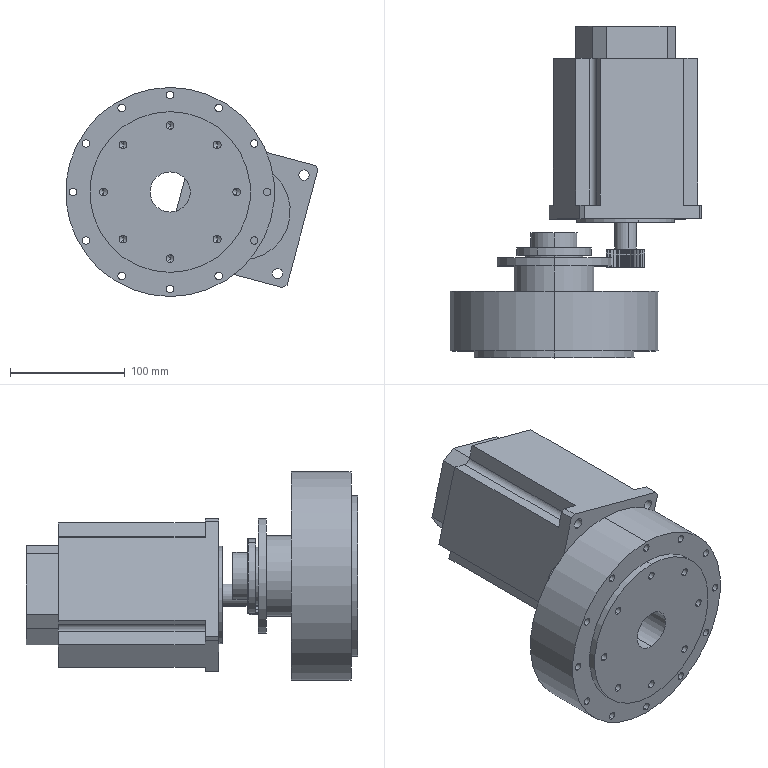Part | SolidWorks | features InContextFeatHolder 6, CompositeCurve 2 | 5 solids | 273 faces | box 219.765 x 289 x 182 mm | volume 3217706 mm3 | cylinder 193 | plane 52 | cone 20 | torus 8 | commonest cylinder face diameters 12.5 x54 28.123 x25 33.75 x25 6.6 x24 6.8 x16 9 x8